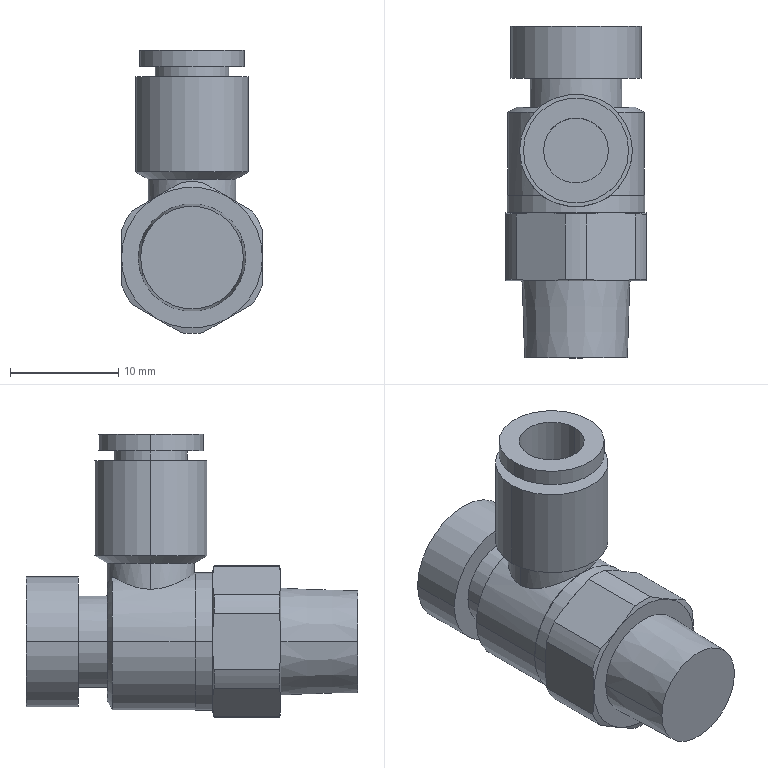Part | STEP file | Speed control valve AS2201F-01-06SA | 1 solid | 61 faces | box 13 x 30.6 x 26.1 mm | volume 3953 mm3 | cylinder 25 | cone 19 | plane 17 | commonest cylinder face diameters 14 x7 6 x2 6.79 x2 8.1 x2 8.45 x2 9.7 x2